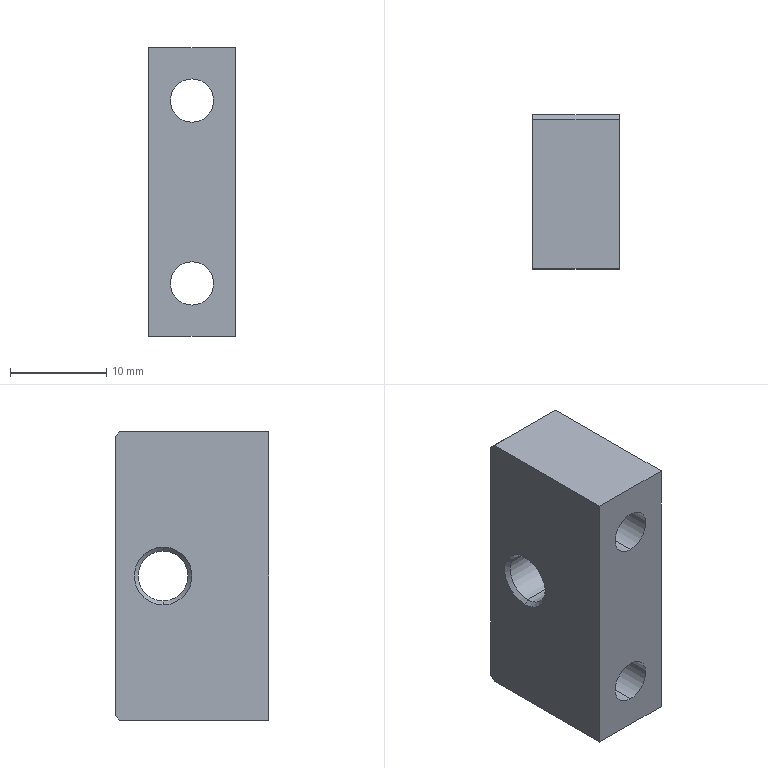Part | STEP file | 001-006-PBP10_M6_H11 | 1 solid | 24 faces | box 9 x 16 x 30 mm | volume 3306 mm3 | cylinder 10 | plane 10 | cone 4 | commonest cylinder face diameters 4.5 x4 8 x4 5.188 x2